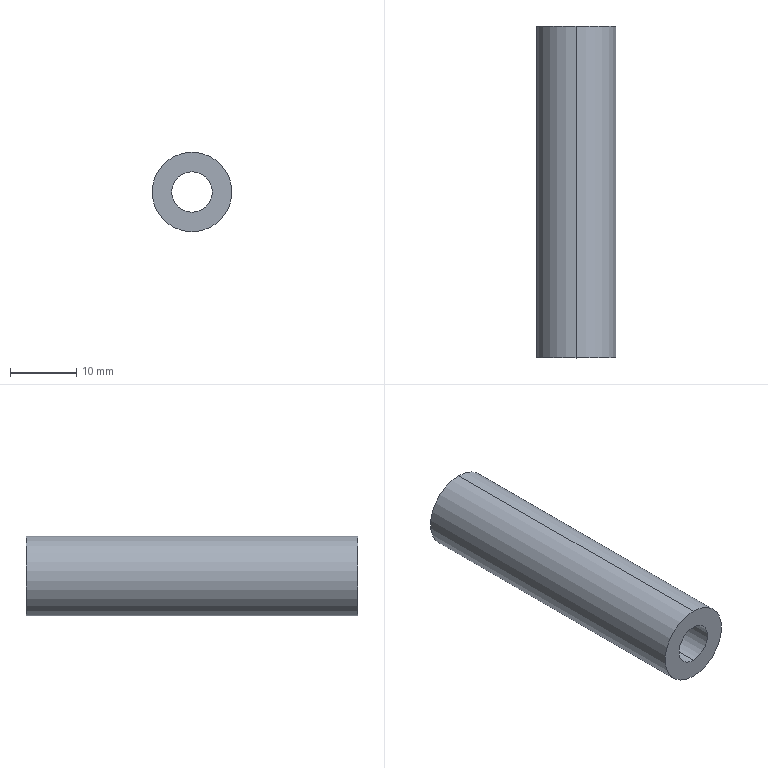Part | SolidWorks | features Extrusion 1 | 1 solid | 6 faces | box 12 x 50 x 12 mm | volume 4194 mm3 | cylinder 4 | plane 2 | commonest cylinder face diameters 6.1 x2 12 x2
STEP:
#1=CARTESIAN_POINT('',(0.,50.,-3.05));
#2=VERTEX_POINT('',#1);
#3=CARTESIAN_POINT('',(0.,50.,3.05));
#4=VERTEX_POINT('',#3);
#5=CARTESIAN_POINT('',(0.,50.,0.));
#6=DIRECTION('',(0.,1.,0.));
#7=DIRECTION('',(0.,0.,1.));
#8=AXIS2_PLACEMENT_3D('',#5,#6,#7);
#9=CIRCLE('',#8,3.05);
#10=EDGE_CURVE('',#2,#4,#9,.T.);
#11=ORIENTED_EDGE('',*,*,#10,.T.);
#12=CARTESIAN_POINT('',(0.,0.,3.05));
#13=VERTEX_POINT('',#12);
#14=CARTESIAN_POINT('',(0.,50.,3.05));
#15=DIRECTION('',(0.,-1.,0.));
#16=VECTOR('',#15,1000.);
#17=LINE('',#14,#16);
#18=EDGE_CURVE('',#4,#13,#17,.T.);
#19=ORIENTED_EDGE('',*,*,#18,.T.);
#20=CARTESIAN_POINT('',(0.,0.,-3.05));
#21=VERTEX_POINT('',#20);
#22=CARTESIAN_POINT('',(0.,0.,0.));
#23=DIRECTION('',(0.,1.,0.));
#24=DIRECTION('',(0.,0.,1.));
#25=AXIS2_PLACEMENT_3D('',#22,#23,#24);
#26=CIRCLE('',#25,3.05);
#27=EDGE_CURVE('',#21,#13,#26,.T.);
#28=ORIENTED_EDGE('',*,*,#27,.F.);
#29=CARTESIAN_POINT('',(0.,50.,-3.05));
#30=DIRECTION('',(0.,-1.,0.));
#31=VECTOR('',#30,1000.);
#32=LINE('',#29,#31);
#33=EDGE_CURVE('',#2,#21,#32,.T.);
#34=ORIENTED_EDGE('',*,*,#33,.F.);
#35=EDGE_LOOP('',(#11,#19,#28,#34));
#36=FACE_OUTER_BOUND('',#35,.T.);
#37=CARTESIAN_POINT('',(0.,50.,0.));
#38=DIRECTION('',(0.,-1.,0.));
#39=DIRECTION('',(0.,0.,-1.));
#40=AXIS2_PLACEMENT_3D('',#37,#38,#39);
#41=CYLINDRICAL_SURFACE('',#40,3.05);
#42=ADVANCED_FACE('',(#36),#41,.F.);
#43=CARTESIAN_POINT('',(0.,50.,6.));
#44=VERTEX_POINT('',#43);
#45=CARTESIAN_POINT('',(0.,50.,-6.));
#46=VERTEX_POINT('',#45);
#47=CARTESIAN_POINT('',(0.,50.,0.));
#48=DIRECTION('',(0.,1.,0.));
#49=DIRECTION('',(0.,0.,1.));
#50=AXIS2_PLACEMENT_3D('',#47,#48,#49);
#51=CIRCLE('',#50,6.);
#52=EDGE_CURVE('',#44,#46,#51,.T.);
#53=ORIENTED_EDGE('',*,*,#52,.F.);
#54=CARTESIAN_POINT('',(0.,0.,6.));
#55=VERTEX_POINT('',#54);
#56=CARTESIAN_POINT('',(0.,50.,6.));
#57=DIRECTION('',(0.,-1.,0.));
#58=VECTOR('',#57,1000.);
#59=LINE('',#56,#58);
#60=EDGE_CURVE('',#44,#55,#59,.T.);
#61=ORIENTED_EDGE('',*,*,#60,.T.);
#62=CARTESIAN_POINT('',(0.,0.,-6.));
#63=VERTEX_POINT('',#62);
#64=CARTESIAN_POINT('',(0.,0.,0.));
#65=DIRECTION('',(0.,1.,0.));
#66=DIRECTION('',(0.,0.,1.));
#67=AXIS2_PLACEMENT_3D('',#64,#65,#66);
#68=CIRCLE('',#67,6.);
#69=EDGE_CURVE('',#55,#63,#68,.T.);
#70=ORIENTED_EDGE('',*,*,#69,.T.);
#71=CARTESIAN_POINT('',(0.,50.,-6.));
#72=DIRECTION('',(0.,-1.,0.));
#73=VECTOR('',#72,1000.);
#74=LINE('',#71,#73);
#75=EDGE_CURVE('',#46,#63,#74,.T.);
#76=ORIENTED_EDGE('',*,*,#75,.F.);
#77=EDGE_LOOP('',(#53,#61,#70,#76));
#78=FACE_OUTER_BOUND('',#77,.T.);
#79=CARTESIAN_POINT('',(0.,50.,0.));
#80=DIRECTION('',(0.,-1.,0.));
#81=DIRECTION('',(0.,0.,-1.));
#82=AXIS2_PLACEMENT_3D('',#79,#80,#81);
#83=CYLINDRICAL_SURFACE('',#82,6.);
#84=ADVANCED_FACE('',(#78),#83,.T.);
#85=CARTESIAN_POINT('',(0.,50.,0.));
#86=DIRECTION('',(0.,1.,0.));
#87=DIRECTION('',(0.,0.,1.));
#88=AXIS2_PLACEMENT_3D('',#85,#86,#87);
#89=CIRCLE('',#88,6.);
#90=EDGE_CURVE('',#46,#44,#89,.T.);
#91=ORIENTED_EDGE('',*,*,#90,.T.);
#92=ORIENTED_EDGE('',*,*,#52,.T.);
#93=EDGE_LOOP('',(#91,#92));
#94=FACE_OUTER_BOUND('',#93,.T.);
#95=ORIENTED_EDGE('',*,*,#10,.F.);
#96=CARTESIAN_POINT('',(0.,50.,0.));
#97=DIRECTION('',(0.,1.,0.));
#98=DIRECTION('',(0.,0.,1.));
#99=AXIS2_PLACEMENT_3D('',#96,#97,#98);
#100=CIRCLE('',#99,3.05);
#101=EDGE_CURVE('',#4,#2,#100,.T.);
#102=ORIENTED_EDGE('',*,*,#101,.F.);
#103=EDGE_LOOP('',(#95,#102));
#104=FACE_BOUND('',#103,.T.);
#105=CARTESIAN_POINT('',(0.,50.,0.));
#106=DIRECTION('',(0.,1.,0.));
#107=DIRECTION('',(0.,0.,1.));
#108=AXIS2_PLACEMENT_3D('',#105,#106,#107);
#109=PLANE('',#108);
#110=ADVANCED_FACE('',(#94,#104),#109,.T.);
#111=CARTESIAN_POINT('',(0.,0.,0.));
#112=DIRECTION('',(0.,1.,0.));
#113=DIRECTION('',(0.,0.,1.));
#114=AXIS2_PLACEMENT_3D('',#111,#112,#113);
#115=CIRCLE('',#114,6.);
#116=EDGE_CURVE('',#63,#55,#115,.T.);
#117=ORIENTED_EDGE('',*,*,#116,.F.);
#118=ORIENTED_EDGE('',*,*,#69,.F.);
#119=EDGE_LOOP('',(#117,#118));
#120=FACE_OUTER_BOUND('',#119,.T.);
#121=ORIENTED_EDGE('',*,*,#27,.T.);
#122=CARTESIAN_POINT('',(0.,0.,0.));
#123=DIRECTION('',(0.,1.,0.));
#124=DIRECTION('',(0.,0.,1.));
#125=AXIS2_PLACEMENT_3D('',#122,#123,#124);
#126=CIRCLE('',#125,3.05);
#127=EDGE_CURVE('',#13,#21,#126,.T.);
#128=ORIENTED_EDGE('',*,*,#127,.T.);
#129=EDGE_LOOP('',(#121,#128));
#130=FACE_BOUND('',#129,.T.);
#131=CARTESIAN_POINT('',(0.,0.,0.));
#132=DIRECTION('',(0.,1.,0.));
#133=DIRECTION('',(0.,0.,1.));
#134=AXIS2_PLACEMENT_3D('',#131,#132,#133);
#135=PLANE('',#134);
#136=ADVANCED_FACE('',(#120,#130),#135,.F.);
#137=ORIENTED_EDGE('',*,*,#60,.F.);
#138=ORIENTED_EDGE('',*,*,#90,.F.);
#139=ORIENTED_EDGE('',*,*,#75,.T.);
#140=ORIENTED_EDGE('',*,*,#116,.T.);
#141=EDGE_LOOP('',(#137,#138,#139,#140));
#142=FACE_OUTER_BOUND('',#141,.T.);
#143=CARTESIAN_POINT('',(0.,50.,0.));
#144=DIRECTION('',(0.,-1.,0.));
#145=DIRECTION('',(0.,0.,-1.));
#146=AXIS2_PLACEMENT_3D('',#143,#144,#145);
#147=CYLINDRICAL_SURFACE('',#146,6.);
#148=ADVANCED_FACE('',(#142),#147,.T.);
#149=ORIENTED_EDGE('',*,*,#18,.F.);
#150=ORIENTED_EDGE('',*,*,#101,.T.);
#151=ORIENTED_EDGE('',*,*,#33,.T.);
#152=ORIENTED_EDGE('',*,*,#127,.F.);
#153=EDGE_LOOP('',(#149,#150,#151,#152));
#154=FACE_OUTER_BOUND('',#153,.T.);
#155=CARTESIAN_POINT('',(0.,50.,0.));
#156=DIRECTION('',(0.,-1.,0.));
#157=DIRECTION('',(0.,0.,-1.));
#158=AXIS2_PLACEMENT_3D('',#155,#156,#157);
#159=CYLINDRICAL_SURFACE('',#158,3.05);
#160=ADVANCED_FACE('',(#154),#159,.F.);
#161=CLOSED_SHELL('',(#42,#84,#110,#136,#148,#160));
#162=MANIFOLD_SOLID_BREP('',#161);
#163=CARTESIAN_POINT('',(0.,0.,0.));
#164=DIRECTION('',(0.,0.,1.));
#165=DIRECTION('',(1.,0.,0.));
#166=AXIS2_PLACEMENT_3D('',#163,#164,#165);
#167=(LENGTH_UNIT()NAMED_UNIT(*)SI_UNIT(.MILLI.,.METRE.));
#168=UNCERTAINTY_MEASURE_WITH_UNIT(LENGTH_MEASURE(0.00001),#167,'','');
#169=(NAMED_UNIT(*)PLANE_ANGLE_UNIT()SI_UNIT($,.RADIAN.));
#170=(NAMED_UNIT(*)SI_UNIT($,.STERADIAN.)SOLID_ANGLE_UNIT());
#171=(GEOMETRIC_REPRESENTATION_CONTEXT(3)GLOBAL_UNCERTAINTY_ASSIGNED_CONTEXT((#168))GLOBAL_UNIT_ASSIGNED_CONTEXT((#167,#169,#170))REPRESENTATION_CONTEXT('',''));
#172=ADVANCED_BREP_SHAPE_REPRESENTATION('',(#162,#166),#171);